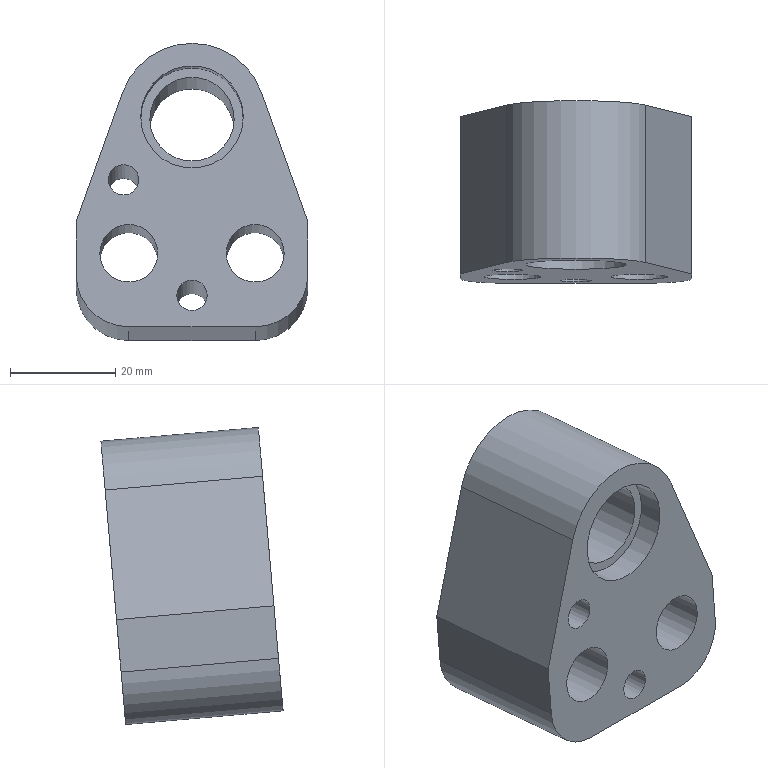Part | NX | features CP-AP 16 2 | 1 solid | 21 faces | box 44 x 34.592 x 56.409 mm | volume 39576 mm3 | cylinder 11 | plane 10 | commonest cylinder face diameters 5.8 x2 11 x2 17 x2 20 x2 16 x1 19.5 x1
STEP:
#1=CARTESIAN_POINT('',(-142.452,-103.656,-62.093));
#2=VERTEX_POINT('',#1);
#3=CARTESIAN_POINT('',(-142.452,-102.784,-52.131));
#4=VERTEX_POINT('',#3);
#5=CARTESIAN_POINT('',(-142.452,-104.527,-72.055));
#6=DIRECTION('',(0.,0.08716,0.9962));
#7=VECTOR('',#6,1000.);
#8=LINE('',#5,#7);
#9=EDGE_CURVE('',#2,#4,#8,.T.);
#10=ORIENTED_EDGE('',*,*,#9,.F.);
#11=CARTESIAN_POINT('',(-142.452,-133.542,-59.478));
#12=VERTEX_POINT('',#11);
#13=CARTESIAN_POINT('',(-142.452,-103.656,-62.093));
#14=DIRECTION('',(0.,-0.9962,0.08716));
#15=VECTOR('',#14,1000.);
#16=LINE('',#13,#15);
#17=EDGE_CURVE('',#2,#12,#16,.T.);
#18=ORIENTED_EDGE('',*,*,#17,.T.);
#19=CARTESIAN_POINT('',(-142.452,-132.67,-49.516));
#20=VERTEX_POINT('',#19);
#21=CARTESIAN_POINT('',(-142.452,-134.413,-69.44));
#22=DIRECTION('',(0.,0.08716,0.9962));
#23=VECTOR('',#22,1000.);
#24=LINE('',#21,#23);
#25=EDGE_CURVE('',#12,#20,#24,.T.);
#26=ORIENTED_EDGE('',*,*,#25,.T.);
#27=CARTESIAN_POINT('',(-142.452,-102.784,-52.131));
#28=DIRECTION('',(0.,-0.9962,0.08716));
#29=VECTOR('',#28,1000.);
#30=LINE('',#27,#29);
#31=EDGE_CURVE('',#4,#20,#30,.T.);
#32=ORIENTED_EDGE('',*,*,#31,.F.);
#33=EDGE_LOOP('',(#10,#18,#26,#32));
#34=FACE_BOUND('',#33,.T.);
#35=CARTESIAN_POINT('',(-142.452,-104.527,-72.055));
#36=DIRECTION('',(1.,0.,0.));
#37=DIRECTION('',(0.,-0.9962,0.08716));
#38=AXIS2_PLACEMENT_3D('',#35,#36,#37);
#39=PLANE('',#38);
#40=ADVANCED_FACE('',(#34),#39,.F.);
#41=CARTESIAN_POINT('',(-133.638,-130.517,-24.906));
#42=VERTEX_POINT('',#41);
#43=CARTESIAN_POINT('',(-142.452,-132.67,-49.516));
#44=DIRECTION('',(0.336,0.08209,0.9383));
#45=VECTOR('',#44,1000.);
#46=LINE('',#43,#45);
#47=EDGE_CURVE('',#20,#42,#46,.T.);
#48=ORIENTED_EDGE('',*,*,#47,.T.);
#49=CARTESIAN_POINT('',(-133.638,-100.631,-27.521));
#50=VERTEX_POINT('',#49);
#51=CARTESIAN_POINT('',(-133.638,-100.631,-27.521));
#52=DIRECTION('',(0.,-0.9962,0.08716));
#53=VECTOR('',#52,1000.);
#54=LINE('',#51,#53);
#55=EDGE_CURVE('',#50,#42,#54,.T.);
#56=ORIENTED_EDGE('',*,*,#55,.F.);
#57=CARTESIAN_POINT('',(-142.452,-102.784,-52.131));
#58=DIRECTION('',(0.336,0.08209,0.9383));
#59=VECTOR('',#58,1000.);
#60=LINE('',#57,#59);
#61=EDGE_CURVE('',#4,#50,#60,.T.);
#62=ORIENTED_EDGE('',*,*,#61,.F.);
#63=ORIENTED_EDGE('',*,*,#31,.T.);
#64=EDGE_LOOP('',(#48,#56,#62,#63));
#65=FACE_BOUND('',#64,.T.);
#66=CARTESIAN_POINT('',(-142.452,-102.784,-52.131));
#67=DIRECTION('',(0.9418,-0.02929,-0.3348));
#68=DIRECTION('',(-0.3359,-0.05278,-0.9404));
#69=AXIS2_PLACEMENT_3D('',#66,#67,#68);
#70=PLANE('',#69);
#71=ADVANCED_FACE('',(#65),#70,.F.);
#72=CARTESIAN_POINT('',(-107.267,-130.517,-24.906));
#73=VERTEX_POINT('',#72);
#74=CARTESIAN_POINT('',(-120.452,-130.927,-29.592));
#75=DIRECTION('',(0.,-0.9962,0.08716));
#76=DIRECTION('',(0.,-0.08716,-0.9962));
#77=AXIS2_PLACEMENT_3D('',#74,#75,#76);
#78=CIRCLE('',#77,14.);
#79=EDGE_CURVE('',#73,#42,#78,.T.);
#80=ORIENTED_EDGE('',*,*,#79,.F.);
#81=CARTESIAN_POINT('',(-107.267,-100.631,-27.521));
#82=VERTEX_POINT('',#81);
#83=CARTESIAN_POINT('',(-107.267,-100.631,-27.521));
#84=DIRECTION('',(0.,-0.9962,0.08716));
#85=VECTOR('',#84,1000.);
#86=LINE('',#83,#85);
#87=EDGE_CURVE('',#82,#73,#86,.T.);
#88=ORIENTED_EDGE('',*,*,#87,.F.);
#89=CARTESIAN_POINT('',(-120.452,-101.041,-32.207));
#90=DIRECTION('',(0.,-0.9962,0.08716));
#91=DIRECTION('',(0.,-0.08716,-0.9962));
#92=AXIS2_PLACEMENT_3D('',#89,#90,#91);
#93=CIRCLE('',#92,14.);
#94=EDGE_CURVE('',#82,#50,#93,.T.);
#95=ORIENTED_EDGE('',*,*,#94,.T.);
#96=ORIENTED_EDGE('',*,*,#55,.T.);
#97=EDGE_LOOP('',(#80,#88,#95,#96));
#98=FACE_BOUND('',#97,.T.);
#99=CARTESIAN_POINT('',(-120.452,-101.041,-32.207));
#100=DIRECTION('',(0.,-0.9962,0.08716));
#101=DIRECTION('',(-1.,0.,0.));
#102=AXIS2_PLACEMENT_3D('',#99,#100,#101);
#103=CYLINDRICAL_SURFACE('',#102,14.);
#104=ADVANCED_FACE('',(#98),#103,.T.);
#105=CARTESIAN_POINT('',(-98.452,-132.67,-49.516));
#106=VERTEX_POINT('',#105);
#107=CARTESIAN_POINT('',(-98.452,-132.67,-49.516));
#108=DIRECTION('',(-0.336,0.08209,0.9383));
#109=VECTOR('',#108,1000.);
#110=LINE('',#107,#109);
#111=EDGE_CURVE('',#106,#73,#110,.T.);
#112=ORIENTED_EDGE('',*,*,#111,.F.);
#113=CARTESIAN_POINT('',(-98.452,-102.784,-52.131));
#114=VERTEX_POINT('',#113);
#115=CARTESIAN_POINT('',(-98.452,-102.784,-52.131));
#116=DIRECTION('',(0.,-0.9962,0.08716));
#117=VECTOR('',#116,1000.);
#118=LINE('',#115,#117);
#119=EDGE_CURVE('',#114,#106,#118,.T.);
#120=ORIENTED_EDGE('',*,*,#119,.F.);
#121=CARTESIAN_POINT('',(-98.452,-102.784,-52.131));
#122=DIRECTION('',(-0.336,0.08209,0.9383));
#123=VECTOR('',#122,1000.);
#124=LINE('',#121,#123);
#125=EDGE_CURVE('',#114,#82,#124,.T.);
#126=ORIENTED_EDGE('',*,*,#125,.T.);
#127=ORIENTED_EDGE('',*,*,#87,.T.);
#128=EDGE_LOOP('',(#112,#120,#126,#127));
#129=FACE_BOUND('',#128,.T.);
#130=CARTESIAN_POINT('',(-98.452,-102.784,-52.131));
#131=DIRECTION('',(0.9418,0.02929,0.3348));
#132=DIRECTION('',(0.3359,-0.1113,-0.9353));
#133=AXIS2_PLACEMENT_3D('',#130,#131,#132);
#134=PLANE('',#133);
#135=ADVANCED_FACE('',(#129),#134,.T.);
#136=CARTESIAN_POINT('',(-98.452,-133.542,-59.478));
#137=VERTEX_POINT('',#136);
#138=CARTESIAN_POINT('',(-98.452,-134.413,-69.44));
#139=DIRECTION('',(0.,0.08716,0.9962));
#140=VECTOR('',#139,1000.);
#141=LINE('',#138,#140);
#142=EDGE_CURVE('',#137,#106,#141,.T.);
#143=ORIENTED_EDGE('',*,*,#142,.F.);
#144=CARTESIAN_POINT('',(-98.452,-103.656,-62.093));
#145=VERTEX_POINT('',#144);
#146=CARTESIAN_POINT('',(-98.452,-103.656,-62.093));
#147=DIRECTION('',(0.,-0.9962,0.08716));
#148=VECTOR('',#147,1000.);
#149=LINE('',#146,#148);
#150=EDGE_CURVE('',#137,#145,#149,.F.);
#151=ORIENTED_EDGE('',*,*,#150,.T.);
#152=CARTESIAN_POINT('',(-98.452,-104.527,-72.055));
#153=DIRECTION('',(0.,0.08716,0.9962));
#154=VECTOR('',#153,1000.);
#155=LINE('',#152,#154);
#156=EDGE_CURVE('',#145,#114,#155,.T.);
#157=ORIENTED_EDGE('',*,*,#156,.T.);
#158=ORIENTED_EDGE('',*,*,#119,.T.);
#159=EDGE_LOOP('',(#143,#151,#157,#158));
#160=FACE_BOUND('',#159,.T.);
#161=CARTESIAN_POINT('',(-98.452,-104.527,-72.055));
#162=DIRECTION('',(1.,0.,0.));
#163=DIRECTION('',(0.,-0.9962,0.08716));
#164=AXIS2_PLACEMENT_3D('',#161,#162,#163);
#165=PLANE('',#164);
#166=ADVANCED_FACE('',(#160),#165,.T.);
#167=CARTESIAN_POINT('',(-108.452,-134.413,-69.44));
#168=VERTEX_POINT('',#167);
#169=CARTESIAN_POINT('',(-132.452,-134.413,-69.44));
#170=VERTEX_POINT('',#169);
#171=CARTESIAN_POINT('',(-98.452,-134.413,-69.44));
#172=DIRECTION('',(-1.,0.,0.));
#173=VECTOR('',#172,1000.);
#174=LINE('',#171,#173);
#175=EDGE_CURVE('',#168,#170,#174,.T.);
#176=ORIENTED_EDGE('',*,*,#175,.T.);
#177=CARTESIAN_POINT('',(-132.452,-104.527,-72.055));
#178=VERTEX_POINT('',#177);
#179=CARTESIAN_POINT('',(-132.452,-104.527,-72.055));
#180=DIRECTION('',(0.,-0.9962,0.08716));
#181=VECTOR('',#180,1000.);
#182=LINE('',#179,#181);
#183=EDGE_CURVE('',#170,#178,#182,.F.);
#184=ORIENTED_EDGE('',*,*,#183,.T.);
#185=CARTESIAN_POINT('',(-108.452,-104.527,-72.055));
#186=VERTEX_POINT('',#185);
#187=CARTESIAN_POINT('',(-98.452,-104.527,-72.055));
#188=DIRECTION('',(-1.,0.,0.));
#189=VECTOR('',#188,1000.);
#190=LINE('',#187,#189);
#191=EDGE_CURVE('',#186,#178,#190,.T.);
#192=ORIENTED_EDGE('',*,*,#191,.F.);
#193=CARTESIAN_POINT('',(-108.452,-134.413,-69.44));
#194=DIRECTION('',(0.,-0.9962,0.08716));
#195=VECTOR('',#194,1000.);
#196=LINE('',#193,#195);
#197=EDGE_CURVE('',#186,#168,#196,.T.);
#198=ORIENTED_EDGE('',*,*,#197,.T.);
#199=EDGE_LOOP('',(#176,#184,#192,#198));
#200=FACE_BOUND('',#199,.T.);
#201=CARTESIAN_POINT('',(-98.452,-104.527,-72.055));
#202=DIRECTION('',(0.,0.08716,0.9962));
#203=DIRECTION('',(0.9962,-0.08682,0.007596));
#204=AXIS2_PLACEMENT_3D('',#201,#202,#203);
#205=PLANE('',#204);
#206=ADVANCED_FACE('',(#200),#205,.F.);
#207=CARTESIAN_POINT('',(-140.952,-103.307,-58.108));
#208=VERTEX_POINT('',#207);
#209=CARTESIAN_POINT('',(-132.452,-103.307,-58.108));
#210=DIRECTION('',(0.,-0.9962,0.08716));
#211=DIRECTION('',(-1.,0.,0.));
#212=AXIS2_PLACEMENT_3D('',#209,#210,#211);
#213=CIRCLE('',#212,8.5);
#214=EDGE_CURVE('',#208,#208,#213,.T.);
#215=ORIENTED_EDGE('',*,*,#214,.T.);
#216=EDGE_LOOP('',(#215));
#217=FACE_BOUND('',#216,.T.);
#218=CARTESIAN_POINT('',(-116.952,-103.307,-58.108));
#219=VERTEX_POINT('',#218);
#220=CARTESIAN_POINT('',(-108.452,-103.307,-58.108));
#221=DIRECTION('',(0.,-0.9962,0.08716));
#222=DIRECTION('',(-1.,0.,0.));
#223=AXIS2_PLACEMENT_3D('',#220,#221,#222);
#224=CIRCLE('',#223,8.5);
#225=EDGE_CURVE('',#219,#219,#224,.T.);
#226=ORIENTED_EDGE('',*,*,#225,.T.);
#227=EDGE_LOOP('',(#226));
#228=FACE_BOUND('',#227,.T.);
#229=CARTESIAN_POINT('',(-136.352,-102.087,-44.161));
#230=VERTEX_POINT('',#229);
#231=CARTESIAN_POINT('',(-133.452,-102.087,-44.161));
#232=DIRECTION('',(0.,-0.9962,0.08716));
#233=DIRECTION('',(-1.,0.,0.));
#234=AXIS2_PLACEMENT_3D('',#231,#232,#233);
#235=CIRCLE('',#234,2.9);
#236=EDGE_CURVE('',#230,#230,#235,.T.);
#237=ORIENTED_EDGE('',*,*,#236,.T.);
#238=EDGE_LOOP('',(#237));
#239=FACE_BOUND('',#238,.T.);
#240=CARTESIAN_POINT('',(-123.352,-104.005,-66.078));
#241=VERTEX_POINT('',#240);
#242=CARTESIAN_POINT('',(-120.452,-104.005,-66.078));
#243=DIRECTION('',(0.,-0.9962,0.08716));
#244=DIRECTION('',(-1.,0.,0.));
#245=AXIS2_PLACEMENT_3D('',#242,#243,#244);
#246=CIRCLE('',#245,2.9);
#247=EDGE_CURVE('',#241,#241,#246,.T.);
#248=ORIENTED_EDGE('',*,*,#247,.T.);
#249=EDGE_LOOP('',(#248));
#250=FACE_BOUND('',#249,.T.);
#251=CARTESIAN_POINT('',(-128.452,-101.041,-32.207));
#252=VERTEX_POINT('',#251);
#253=CARTESIAN_POINT('',(-120.452,-101.041,-32.207));
#254=DIRECTION('',(0.,-0.9962,0.08716));
#255=DIRECTION('',(-1.,0.,0.));
#256=AXIS2_PLACEMENT_3D('',#253,#254,#255);
#257=CIRCLE('',#256,8.);
#258=EDGE_CURVE('',#252,#252,#257,.T.);
#259=ORIENTED_EDGE('',*,*,#258,.T.);
#260=EDGE_LOOP('',(#259));
#261=FACE_BOUND('',#260,.T.);
#262=ORIENTED_EDGE('',*,*,#191,.T.);
#263=CARTESIAN_POINT('',(-132.452,-103.656,-62.093));
#264=DIRECTION('',(0.,-0.9962,0.08716));
#265=DIRECTION('',(-1.,0.,0.));
#266=AXIS2_PLACEMENT_3D('',#263,#264,#265);
#267=CIRCLE('',#266,10.);
#268=EDGE_CURVE('',#178,#2,#267,.F.);
#269=ORIENTED_EDGE('',*,*,#268,.T.);
#270=ORIENTED_EDGE('',*,*,#9,.T.);
#271=ORIENTED_EDGE('',*,*,#61,.T.);
#272=ORIENTED_EDGE('',*,*,#94,.F.);
#273=ORIENTED_EDGE('',*,*,#125,.F.);
#274=ORIENTED_EDGE('',*,*,#156,.F.);
#275=CARTESIAN_POINT('',(-108.452,-103.656,-62.093));
#276=DIRECTION('',(0.,-0.9962,0.08716));
#277=DIRECTION('',(-1.,0.,0.));
#278=AXIS2_PLACEMENT_3D('',#275,#276,#277);
#279=CIRCLE('',#278,10.);
#280=EDGE_CURVE('',#145,#186,#279,.F.);
#281=ORIENTED_EDGE('',*,*,#280,.T.);
#282=EDGE_LOOP('',(#262,#269,#270,#271,#272,#273,#274,#281));
#283=FACE_BOUND('',#282,.T.);
#284=CARTESIAN_POINT('',(-120.452,-101.041,-32.207));
#285=DIRECTION('',(0.,-0.9962,0.08716));
#286=DIRECTION('',(-1.,0.,0.));
#287=AXIS2_PLACEMENT_3D('',#284,#285,#286);
#288=PLANE('',#287);
#289=ADVANCED_FACE('',(#217,#228,#239,#250,#261,#283),#288,.F.);
#290=CARTESIAN_POINT('',(-137.952,-133.193,-55.494));
#291=VERTEX_POINT('',#290);
#292=CARTESIAN_POINT('',(-132.452,-133.193,-55.494));
#293=DIRECTION('',(0.,-0.9962,0.08716));
#294=DIRECTION('',(-1.,0.,0.));
#295=AXIS2_PLACEMENT_3D('',#292,#293,#294);
#296=CIRCLE('',#295,5.5);
#297=EDGE_CURVE('',#291,#291,#296,.T.);
#298=ORIENTED_EDGE('',*,*,#297,.F.);
#299=EDGE_LOOP('',(#298));
#300=FACE_BOUND('',#299,.T.);
#301=CARTESIAN_POINT('',(-113.952,-133.193,-55.494));
#302=VERTEX_POINT('',#301);
#303=CARTESIAN_POINT('',(-108.452,-133.193,-55.494));
#304=DIRECTION('',(0.,-0.9962,0.08716));
#305=DIRECTION('',(-1.,0.,0.));
#306=AXIS2_PLACEMENT_3D('',#303,#304,#305);
#307=CIRCLE('',#306,5.5);
#308=EDGE_CURVE('',#302,#302,#307,.T.);
#309=ORIENTED_EDGE('',*,*,#308,.F.);
#310=EDGE_LOOP('',(#309));
#311=FACE_BOUND('',#310,.T.);
#312=CARTESIAN_POINT('',(-136.352,-131.973,-41.547));
#313=VERTEX_POINT('',#312);
#314=CARTESIAN_POINT('',(-133.452,-131.973,-41.547));
#315=DIRECTION('',(0.,-0.9962,0.08716));
#316=DIRECTION('',(-1.,0.,0.));
#317=AXIS2_PLACEMENT_3D('',#314,#315,#316);
#318=CIRCLE('',#317,2.9);
#319=EDGE_CURVE('',#313,#313,#318,.T.);
#320=ORIENTED_EDGE('',*,*,#319,.F.);
#321=EDGE_LOOP('',(#320));
#322=FACE_BOUND('',#321,.T.);
#323=CARTESIAN_POINT('',(-123.352,-133.89,-63.463));
#324=VERTEX_POINT('',#323);
#325=CARTESIAN_POINT('',(-120.452,-133.89,-63.463));
#326=DIRECTION('',(0.,-0.9962,0.08716));
#327=DIRECTION('',(-1.,0.,0.));
#328=AXIS2_PLACEMENT_3D('',#325,#326,#327);
#329=CIRCLE('',#328,2.9);
#330=EDGE_CURVE('',#324,#324,#329,.T.);
#331=ORIENTED_EDGE('',*,*,#330,.F.);
#332=EDGE_LOOP('',(#331));
#333=FACE_BOUND('',#332,.T.);
#334=CARTESIAN_POINT('',(-130.202,-130.927,-29.592));
#335=VERTEX_POINT('',#334);
#336=CARTESIAN_POINT('',(-120.452,-130.927,-29.592));
#337=DIRECTION('',(0.,-0.9962,0.08716));
#338=DIRECTION('',(-1.,0.,0.));
#339=AXIS2_PLACEMENT_3D('',#336,#337,#338);
#340=CIRCLE('',#339,9.75);
#341=EDGE_CURVE('',#335,#335,#340,.T.);
#342=ORIENTED_EDGE('',*,*,#341,.F.);
#343=EDGE_LOOP('',(#342));
#344=FACE_BOUND('',#343,.T.);
#345=ORIENTED_EDGE('',*,*,#25,.F.);
#346=CARTESIAN_POINT('',(-132.452,-133.542,-59.478));
#347=DIRECTION('',(0.,-0.9962,0.08716));
#348=DIRECTION('',(-1.,0.,0.));
#349=AXIS2_PLACEMENT_3D('',#346,#347,#348);
#350=CIRCLE('',#349,10.);
#351=EDGE_CURVE('',#12,#170,#350,.T.);
#352=ORIENTED_EDGE('',*,*,#351,.T.);
#353=ORIENTED_EDGE('',*,*,#175,.F.);
#354=CARTESIAN_POINT('',(-108.452,-133.542,-59.478));
#355=DIRECTION('',(0.,-0.9962,0.08716));
#356=DIRECTION('',(-1.,0.,0.));
#357=AXIS2_PLACEMENT_3D('',#354,#355,#356);
#358=CIRCLE('',#357,10.);
#359=EDGE_CURVE('',#168,#137,#358,.T.);
#360=ORIENTED_EDGE('',*,*,#359,.T.);
#361=ORIENTED_EDGE('',*,*,#142,.T.);
#362=ORIENTED_EDGE('',*,*,#111,.T.);
#363=ORIENTED_EDGE('',*,*,#79,.T.);
#364=ORIENTED_EDGE('',*,*,#47,.F.);
#365=EDGE_LOOP('',(#345,#352,#353,#360,#361,#362,#363,#364));
#366=FACE_BOUND('',#365,.T.);
#367=CARTESIAN_POINT('',(-120.452,-130.927,-29.592));
#368=DIRECTION('',(0.,-0.9962,0.08716));
#369=DIRECTION('',(-1.,0.,0.));
#370=AXIS2_PLACEMENT_3D('',#367,#368,#369);
#371=PLANE('',#370);
#372=ADVANCED_FACE('',(#300,#311,#322,#333,#344,#366),#371,.T.);
#373=ORIENTED_EDGE('',*,*,#280,.F.);
#374=ORIENTED_EDGE('',*,*,#150,.F.);
#375=ORIENTED_EDGE('',*,*,#359,.F.);
#376=ORIENTED_EDGE('',*,*,#197,.F.);
#377=EDGE_LOOP('',(#373,#374,#375,#376));
#378=FACE_BOUND('',#377,.T.);
#379=CARTESIAN_POINT('',(-108.452,-103.656,-62.093));
#380=DIRECTION('',(0.,0.9962,-0.08716));
#381=DIRECTION('',(1.,0.,0.));
#382=AXIS2_PLACEMENT_3D('',#379,#380,#381);
#383=CYLINDRICAL_SURFACE('',#382,10.);
#384=ADVANCED_FACE('',(#378),#383,.T.);
#385=ORIENTED_EDGE('',*,*,#268,.F.);
#386=ORIENTED_EDGE('',*,*,#183,.F.);
#387=ORIENTED_EDGE('',*,*,#351,.F.);
#388=ORIENTED_EDGE('',*,*,#17,.F.);
#389=EDGE_LOOP('',(#385,#386,#387,#388));
#390=FACE_BOUND('',#389,.T.);
#391=CARTESIAN_POINT('',(-132.452,-103.656,-62.093));
#392=DIRECTION('',(0.,-0.9962,0.08716));
#393=DIRECTION('',(-1.,0.,0.));
#394=AXIS2_PLACEMENT_3D('',#391,#392,#393);
#395=CYLINDRICAL_SURFACE('',#394,10.);
#396=ADVANCED_FACE('',(#390),#395,.T.);
#397=CARTESIAN_POINT('',(-112.452,-125.946,-30.028));
#398=VERTEX_POINT('',#397);
#399=CARTESIAN_POINT('',(-120.452,-125.946,-30.028));
#400=DIRECTION('',(0.,0.9962,-0.08716));
#401=DIRECTION('',(1.,0.,0.));
#402=AXIS2_PLACEMENT_3D('',#399,#400,#401);
#403=CIRCLE('',#402,8.);
#404=EDGE_CURVE('',#398,#398,#403,.T.);
#405=ORIENTED_EDGE('',*,*,#404,.T.);
#406=EDGE_LOOP('',(#405));
#407=FACE_BOUND('',#406,.T.);
#408=CARTESIAN_POINT('',(-130.202,-125.946,-30.028));
#409=VERTEX_POINT('',#408);
#410=CARTESIAN_POINT('',(-120.452,-125.946,-30.028));
#411=DIRECTION('',(0.,-0.9962,0.08716));
#412=DIRECTION('',(-1.,0.,0.));
#413=AXIS2_PLACEMENT_3D('',#410,#411,#412);
#414=CIRCLE('',#413,9.75);
#415=EDGE_CURVE('',#409,#409,#414,.T.);
#416=ORIENTED_EDGE('',*,*,#415,.T.);
#417=EDGE_LOOP('',(#416));
#418=FACE_BOUND('',#417,.T.);
#419=CARTESIAN_POINT('',(-120.452,-125.946,-30.028));
#420=DIRECTION('',(0.,0.9962,-0.08716));
#421=DIRECTION('',(1.,0.,0.));
#422=AXIS2_PLACEMENT_3D('',#419,#420,#421);
#423=PLANE('',#422);
#424=ADVANCED_FACE('',(#407,#418),#423,.F.);
#425=ORIENTED_EDGE('',*,*,#341,.T.);
#426=EDGE_LOOP('',(#425));
#427=FACE_BOUND('',#426,.T.);
#428=ORIENTED_EDGE('',*,*,#415,.F.);
#429=EDGE_LOOP('',(#428));
#430=FACE_BOUND('',#429,.T.);
#431=CARTESIAN_POINT('',(-120.452,-131.923,-29.505));
#432=DIRECTION('',(0.,0.9962,-0.08716));
#433=DIRECTION('',(1.,0.,0.));
#434=AXIS2_PLACEMENT_3D('',#431,#432,#433);
#435=CYLINDRICAL_SURFACE('',#434,9.75);
#436=ADVANCED_FACE('',(#427,#430),#435,.F.);
#437=ORIENTED_EDGE('',*,*,#404,.F.);
#438=EDGE_LOOP('',(#437));
#439=FACE_BOUND('',#438,.T.);
#440=ORIENTED_EDGE('',*,*,#258,.F.);
#441=EDGE_LOOP('',(#440));
#442=FACE_BOUND('',#441,.T.);
#443=CARTESIAN_POINT('',(-120.452,-131.923,-29.505));
#444=DIRECTION('',(0.,0.9962,-0.08716));
#445=DIRECTION('',(1.,0.,0.));
#446=AXIS2_PLACEMENT_3D('',#443,#444,#445);
#447=CYLINDRICAL_SURFACE('',#446,8.);
#448=ADVANCED_FACE('',(#439,#442),#447,.F.);
#449=ORIENTED_EDGE('',*,*,#330,.T.);
#450=EDGE_LOOP('',(#449));
#451=FACE_BOUND('',#450,.T.);
#452=ORIENTED_EDGE('',*,*,#247,.F.);
#453=EDGE_LOOP('',(#452));
#454=FACE_BOUND('',#453,.T.);
#455=CARTESIAN_POINT('',(-120.452,-134.887,-63.376));
#456=DIRECTION('',(0.,0.9962,-0.08716));
#457=DIRECTION('',(1.,0.,0.));
#458=AXIS2_PLACEMENT_3D('',#455,#456,#457);
#459=CYLINDRICAL_SURFACE('',#458,2.9);
#460=ADVANCED_FACE('',(#451,#454),#459,.F.);
#461=ORIENTED_EDGE('',*,*,#319,.T.);
#462=EDGE_LOOP('',(#461));
#463=FACE_BOUND('',#462,.T.);
#464=ORIENTED_EDGE('',*,*,#236,.F.);
#465=EDGE_LOOP('',(#464));
#466=FACE_BOUND('',#465,.T.);
#467=CARTESIAN_POINT('',(-133.452,-132.969,-41.46));
#468=DIRECTION('',(0.,0.9962,-0.08716));
#469=DIRECTION('',(1.,0.,0.));
#470=AXIS2_PLACEMENT_3D('',#467,#468,#469);
#471=CYLINDRICAL_SURFACE('',#470,2.9);
#472=ADVANCED_FACE('',(#463,#466),#471,.F.);
#473=CARTESIAN_POINT('',(-113.952,-115.262,-57.062));
#474=VERTEX_POINT('',#473);
#475=CARTESIAN_POINT('',(-108.452,-115.262,-57.062));
#476=DIRECTION('',(0.,-0.9962,0.08716));
#477=DIRECTION('',(-1.,0.,0.));
#478=AXIS2_PLACEMENT_3D('',#475,#476,#477);
#479=CIRCLE('',#478,5.5);
#480=EDGE_CURVE('',#474,#474,#479,.F.);
#481=ORIENTED_EDGE('',*,*,#480,.T.);
#482=EDGE_LOOP('',(#481));
#483=FACE_BOUND('',#482,.T.);
#484=ORIENTED_EDGE('',*,*,#308,.T.);
#485=EDGE_LOOP('',(#484));
#486=FACE_BOUND('',#485,.T.);
#487=CARTESIAN_POINT('',(-108.452,-134.189,-55.406));
#488=DIRECTION('',(0.,0.9962,-0.08716));
#489=DIRECTION('',(1.,0.,0.));
#490=AXIS2_PLACEMENT_3D('',#487,#488,#489);
#491=CYLINDRICAL_SURFACE('',#490,5.5);
#492=ADVANCED_FACE('',(#483,#486),#491,.F.);
#493=CARTESIAN_POINT('',(-137.952,-115.262,-57.062));
#494=VERTEX_POINT('',#493);
#495=CARTESIAN_POINT('',(-132.452,-115.262,-57.062));
#496=DIRECTION('',(0.,-0.9962,0.08716));
#497=DIRECTION('',(-1.,0.,0.));
#498=AXIS2_PLACEMENT_3D('',#495,#496,#497);
#499=CIRCLE('',#498,5.5);
#500=EDGE_CURVE('',#494,#494,#499,.F.);
#501=ORIENTED_EDGE('',*,*,#500,.T.);
#502=EDGE_LOOP('',(#501));
#503=FACE_BOUND('',#502,.T.);
#504=ORIENTED_EDGE('',*,*,#297,.T.);
#505=EDGE_LOOP('',(#504));
#506=FACE_BOUND('',#505,.T.);
#507=CARTESIAN_POINT('',(-132.452,-134.189,-55.406));
#508=DIRECTION('',(0.,0.9962,-0.08716));
#509=DIRECTION('',(1.,0.,0.));
#510=AXIS2_PLACEMENT_3D('',#507,#508,#509);
#511=CYLINDRICAL_SURFACE('',#510,5.5);
#512=ADVANCED_FACE('',(#503,#506),#511,.F.);
#513=CARTESIAN_POINT('',(-99.952,-115.262,-57.062));
#514=VERTEX_POINT('',#513);
#515=CARTESIAN_POINT('',(-108.452,-115.262,-57.062));
#516=DIRECTION('',(0.,0.9962,-0.08716));
#517=DIRECTION('',(1.,0.,0.));
#518=AXIS2_PLACEMENT_3D('',#515,#516,#517);
#519=CIRCLE('',#518,8.5);
#520=EDGE_CURVE('',#514,#514,#519,.T.);
#521=ORIENTED_EDGE('',*,*,#520,.F.);
#522=EDGE_LOOP('',(#521));
#523=FACE_BOUND('',#522,.T.);
#524=ORIENTED_EDGE('',*,*,#225,.F.);
#525=EDGE_LOOP('',(#524));
#526=FACE_BOUND('',#525,.T.);
#527=CARTESIAN_POINT('',(-108.452,-115.262,-57.062));
#528=DIRECTION('',(0.,0.9962,-0.08716));
#529=DIRECTION('',(1.,0.,0.));
#530=AXIS2_PLACEMENT_3D('',#527,#528,#529);
#531=CYLINDRICAL_SURFACE('',#530,8.5);
#532=ADVANCED_FACE('',(#523,#526),#531,.F.);
#533=ORIENTED_EDGE('',*,*,#520,.T.);
#534=EDGE_LOOP('',(#533));
#535=FACE_BOUND('',#534,.T.);
#536=ORIENTED_EDGE('',*,*,#480,.F.);
#537=EDGE_LOOP('',(#536));
#538=FACE_BOUND('',#537,.T.);
#539=CARTESIAN_POINT('',(-108.452,-115.262,-57.062));
#540=DIRECTION('',(0.,-0.9962,0.08716));
#541=DIRECTION('',(-1.,0.,0.));
#542=AXIS2_PLACEMENT_3D('',#539,#540,#541);
#543=PLANE('',#542);
#544=ADVANCED_FACE('',(#535,#538),#543,.F.);
#545=CARTESIAN_POINT('',(-123.952,-115.262,-57.062));
#546=VERTEX_POINT('',#545);
#547=CARTESIAN_POINT('',(-132.452,-115.262,-57.062));
#548=DIRECTION('',(0.,0.9962,-0.08716));
#549=DIRECTION('',(1.,0.,0.));
#550=AXIS2_PLACEMENT_3D('',#547,#548,#549);
#551=CIRCLE('',#550,8.5);
#552=EDGE_CURVE('',#546,#546,#551,.T.);
#553=ORIENTED_EDGE('',*,*,#552,.F.);
#554=EDGE_LOOP('',(#553));
#555=FACE_BOUND('',#554,.T.);
#556=ORIENTED_EDGE('',*,*,#214,.F.);
#557=EDGE_LOOP('',(#556));
#558=FACE_BOUND('',#557,.T.);
#559=CARTESIAN_POINT('',(-132.452,-115.262,-57.062));
#560=DIRECTION('',(0.,0.9962,-0.08716));
#561=DIRECTION('',(1.,0.,0.));
#562=AXIS2_PLACEMENT_3D('',#559,#560,#561);
#563=CYLINDRICAL_SURFACE('',#562,8.5);
#564=ADVANCED_FACE('',(#555,#558),#563,.F.);
#565=ORIENTED_EDGE('',*,*,#552,.T.);
#566=EDGE_LOOP('',(#565));
#567=FACE_BOUND('',#566,.T.);
#568=ORIENTED_EDGE('',*,*,#500,.F.);
#569=EDGE_LOOP('',(#568));
#570=FACE_BOUND('',#569,.T.);
#571=CARTESIAN_POINT('',(-132.452,-115.262,-57.062));
#572=DIRECTION('',(0.,-0.9962,0.08716));
#573=DIRECTION('',(-1.,0.,0.));
#574=AXIS2_PLACEMENT_3D('',#571,#572,#573);
#575=PLANE('',#574);
#576=ADVANCED_FACE('',(#567,#570),#575,.F.);
#577=CLOSED_SHELL('',(#40,#71,#104,#135,#166,#206,#289,#372,#384,#396,#424,#436,#448,#460,#472,#492,#512,#532,#544,#564,#576));
#578=MANIFOLD_SOLID_BREP('',#577);
#579=(LENGTH_UNIT()NAMED_UNIT(*)SI_UNIT(.MILLI.,.METRE.));
#580=UNCERTAINTY_MEASURE_WITH_UNIT(LENGTH_MEASURE(0.00001),#579,'','');
#581=(NAMED_UNIT(*)PLANE_ANGLE_UNIT()SI_UNIT($,.RADIAN.));
#582=(NAMED_UNIT(*)SI_UNIT($,.STERADIAN.)SOLID_ANGLE_UNIT());
#583=(GEOMETRIC_REPRESENTATION_CONTEXT(3)GLOBAL_UNCERTAINTY_ASSIGNED_CONTEXT((#580))GLOBAL_UNIT_ASSIGNED_CONTEXT((#579,#581,#582))REPRESENTATION_CONTEXT('',''));
#584=ADVANCED_BREP_SHAPE_REPRESENTATION('',(#578),#583);